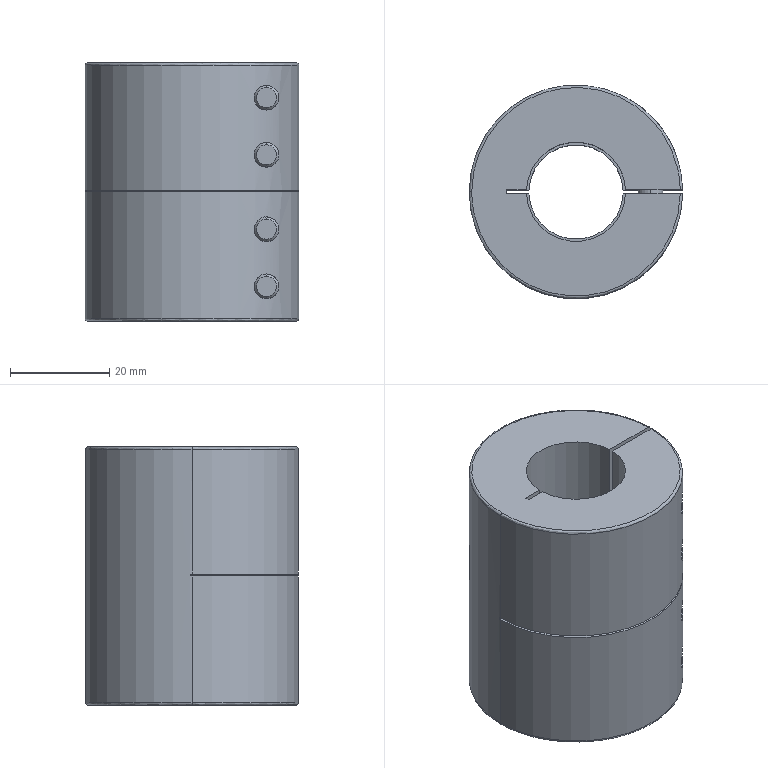Part | SolidWorks | features BaseBody 1 | 1 solid | 142 faces | box 42.996 x 43 x 52 mm | volume 57062 mm3 | plane 64 | cylinder 58 | cone 16 | spline 4 | commonest cylinder face diameters 5 x16 5.4 x16 8.35 x8 8.75 x8 22.3 x3 43 x3